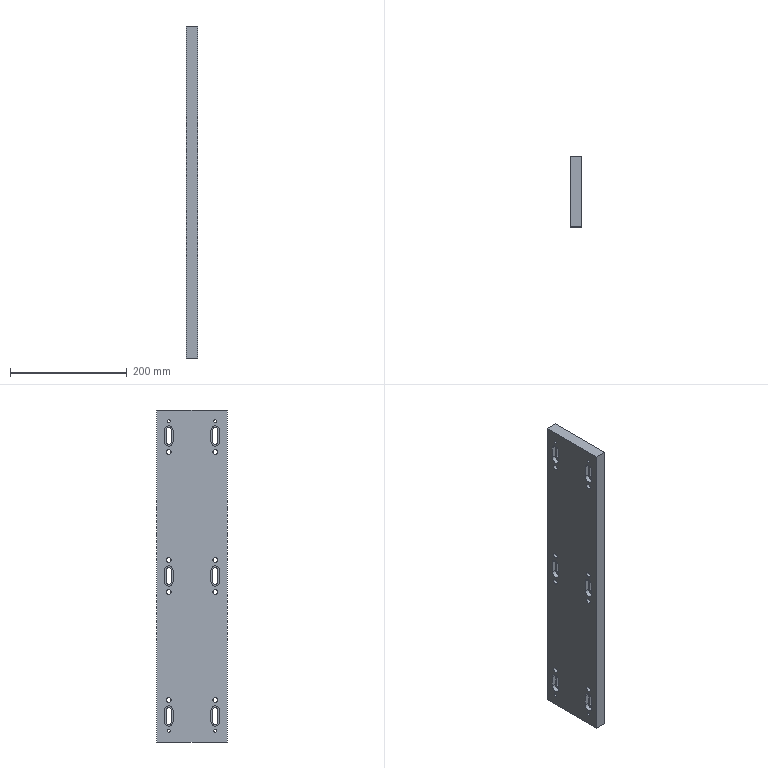Part | NX | 1 solid | 72 faces | box 20 x 120 x 569 mm | volume 1314527 mm3 | cylinder 36 | plane 36 | commonest cylinder face diameters 9 x12 15 x12 8.5 x8 5 x4